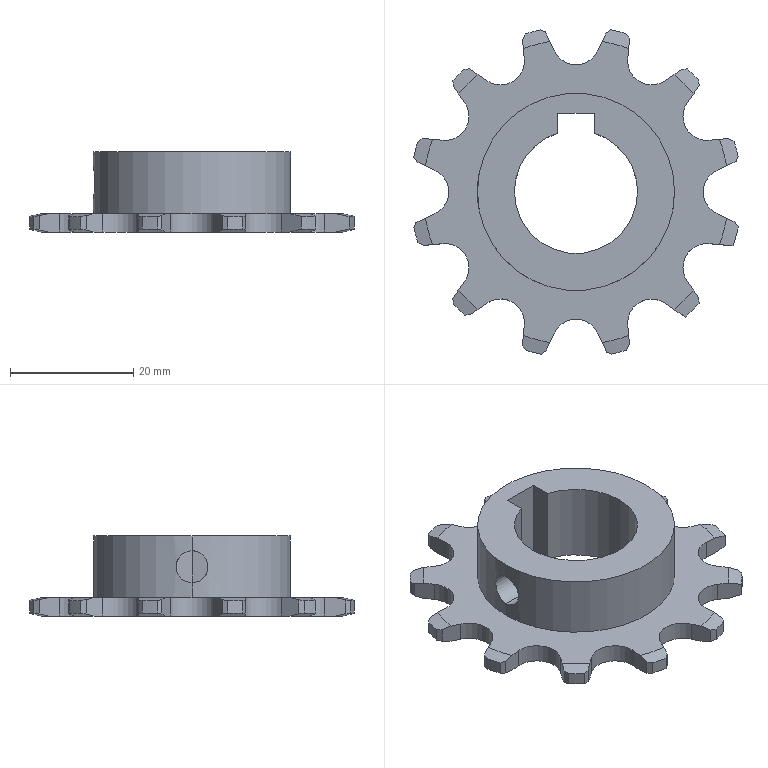Part | NX | features BREP 1 | 1 solid | 112 faces | box 52.696 x 52.696 x 13 mm | volume 8744 mm3 | plane 52 | cylinder 36 | cone 24 | commonest cylinder face diameters 7.77 x17 53.9 x12 20 x3 5.2 x2 32 x2